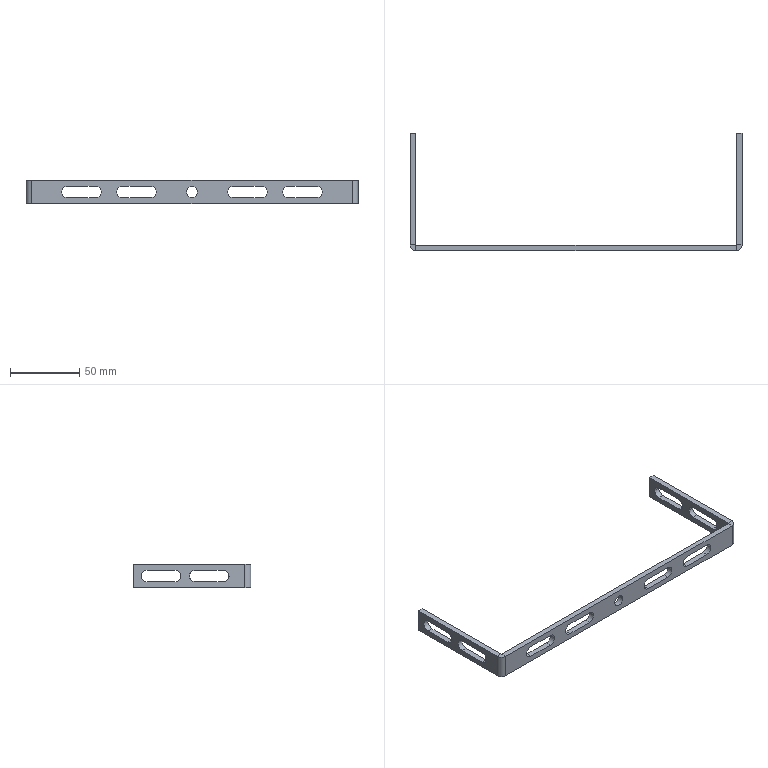Part | SolidWorks | features ICE 3, FlatPattern 1, MirrorPattern 1, SMBaseFlange 1, SheetMetal 1 | 1 solid | 60 faces | box 240 x 85 x 17 mm | volume 19751 mm3 | plane 34 | cylinder 26 | commonest cylinder face diameters 8.5 x20 0.4 x2 8 x2 8.4 x2